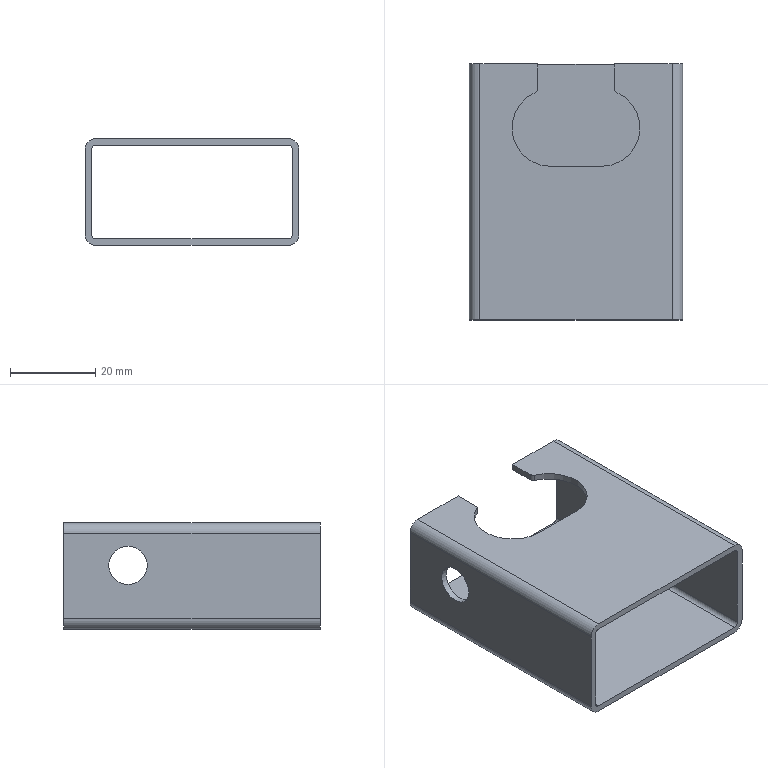Part | STEP file | Q7C0508 | 1 solid | 27 faces | box 50 x 60 x 25 mm | volume 11629 mm3 | cylinder 14 | plane 13 | commonest cylinder face diameters 2 x6 5 x4 9 x2 18 x2